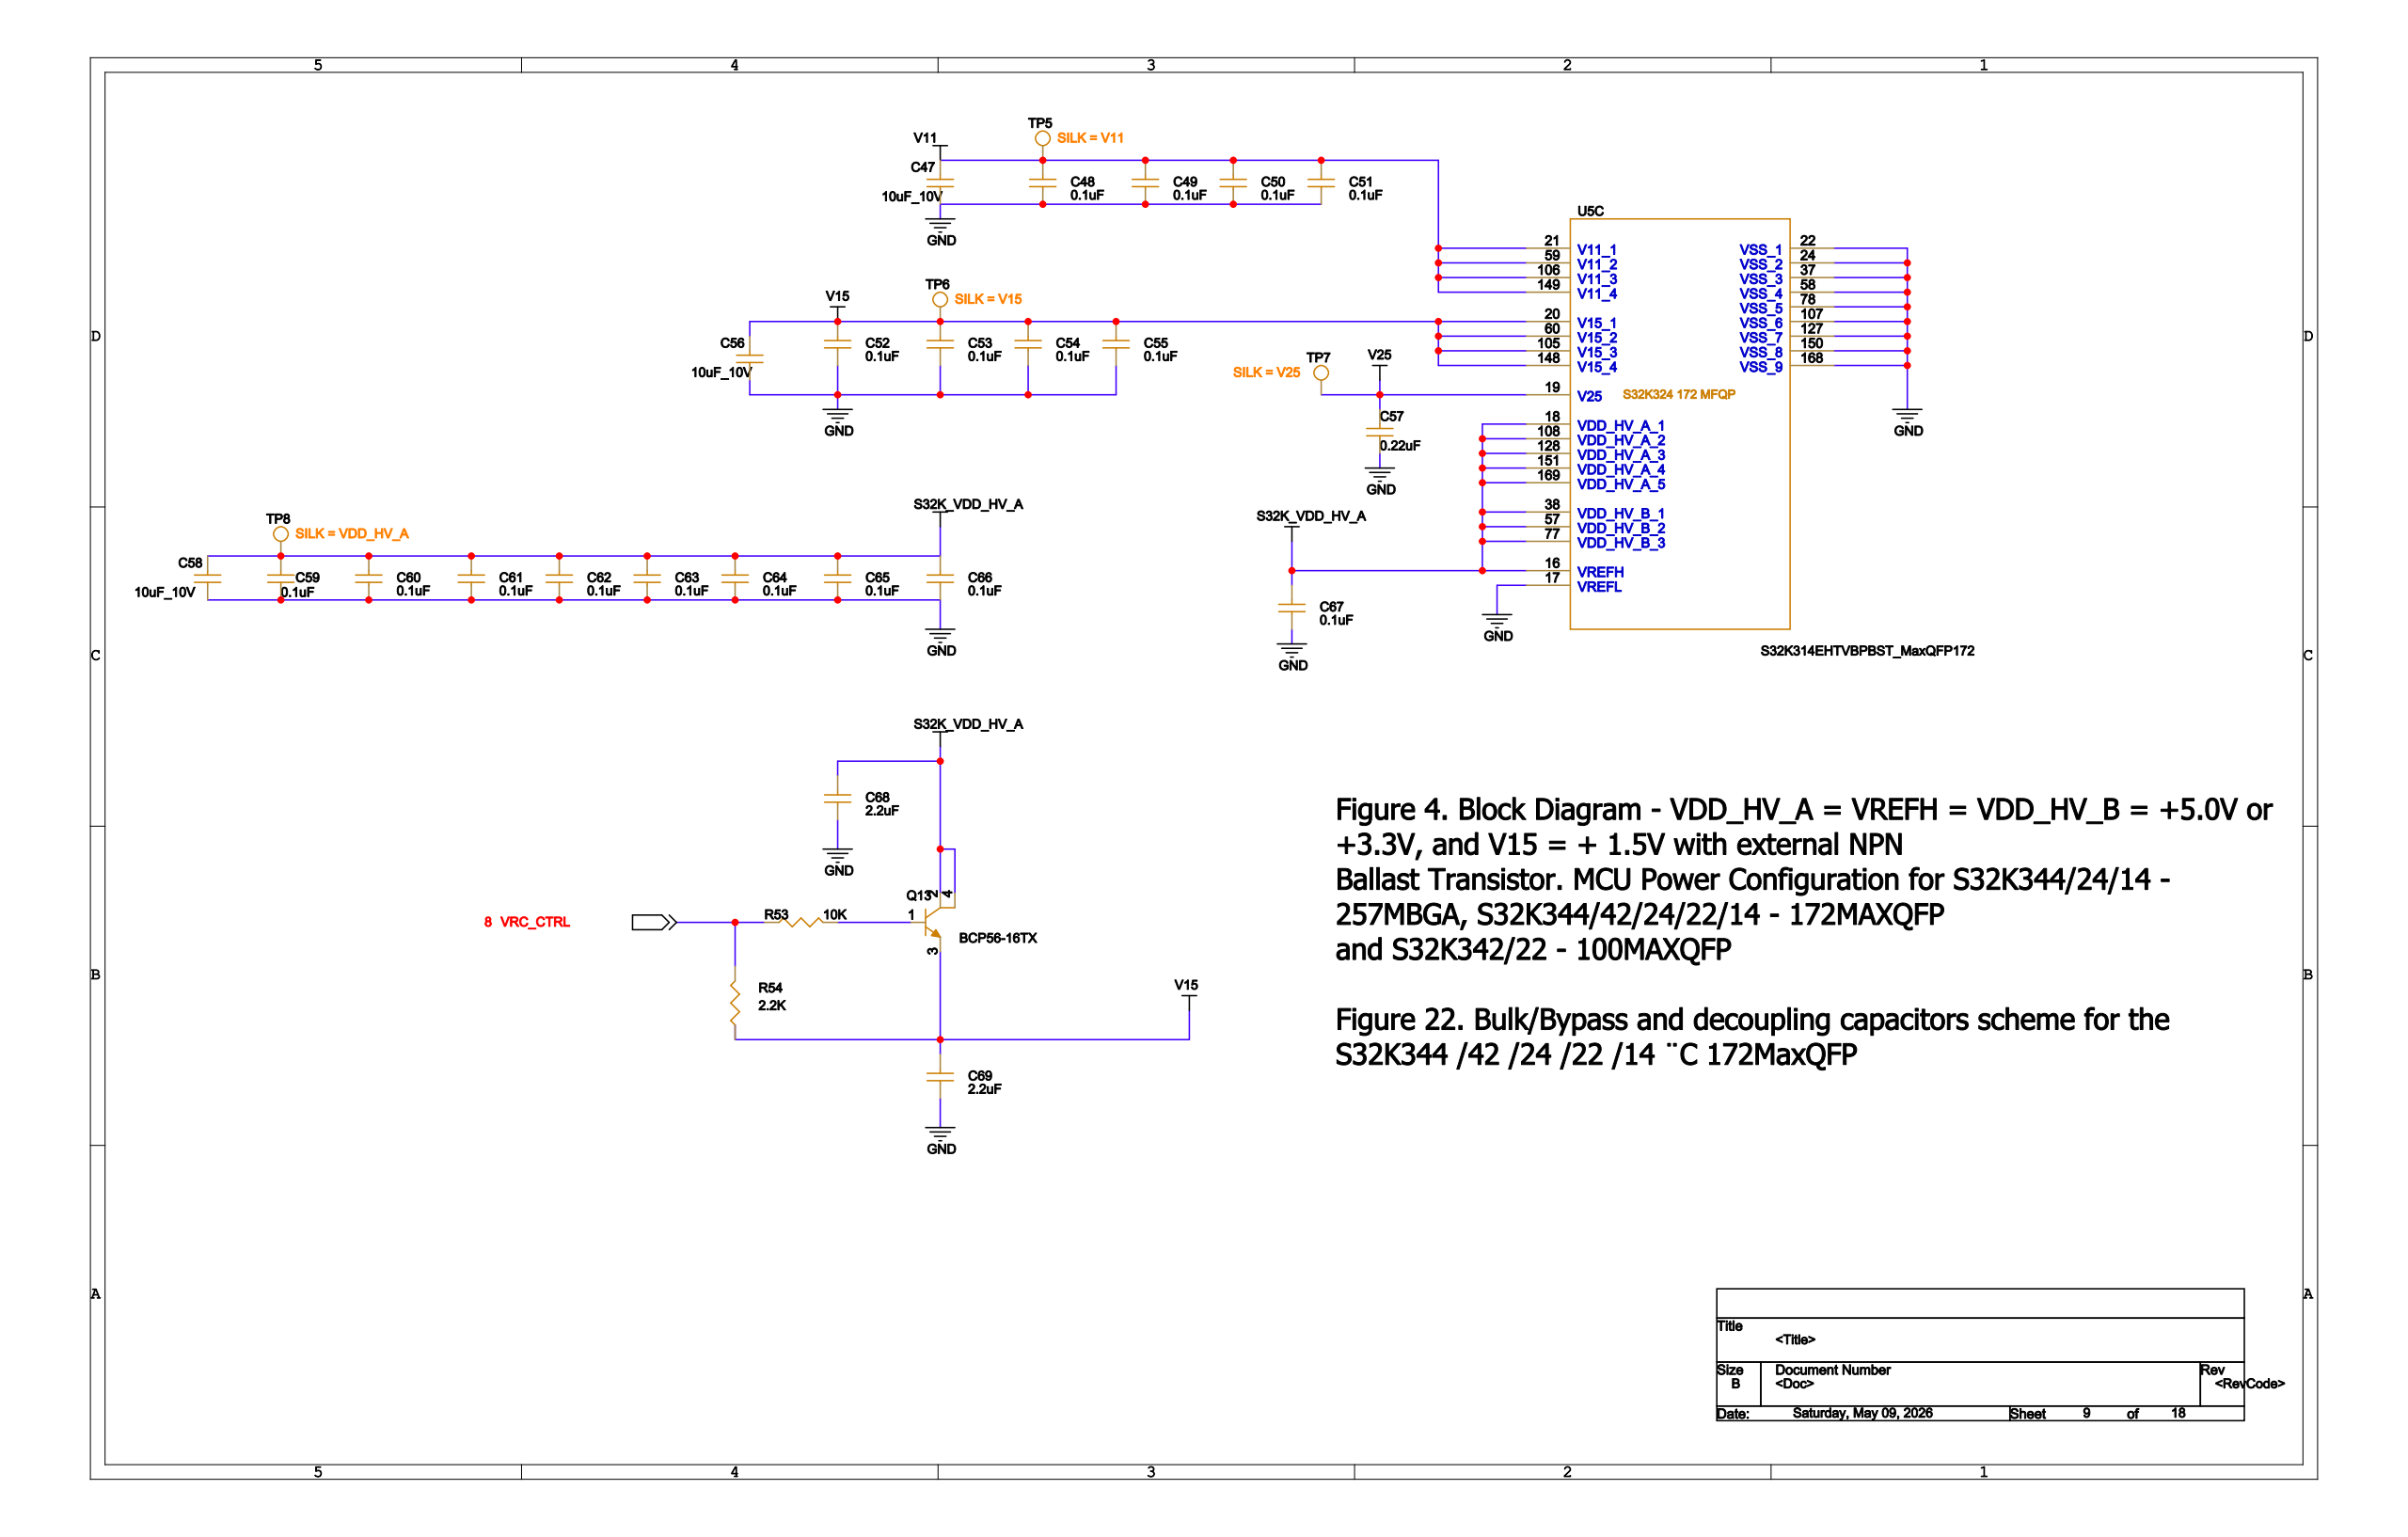Circuit board | Cadence Allegro | 330 parts | 215 nets | one sheet of the schematic
Parts on this sheet (reference | value | footprint):
C47 | 10uF_10V | 0603
C48 | 0.1uF | 0402
C49 | 0.1uF | 0402
C50 | 0.1uF | 0402
C51 | 0.1uF | 0402
C52 | 0.1uF | 0402
C53 | 0.1uF | 0402
C54 | 0.1uF | 0402
C55 | 0.1uF | 0402
C56 | 10uF_10V | 0603
C57 | 0.22uF | 0402
C58 | 10uF_10V | 0603
C59 | 0.1uF | 0402
C60 | 0.1uF | 0402
C61 | 0.1uF | 0402
C62 | 0.1uF | 0402
C63 | 0.1uF | 0402
C64 | 0.1uF | 0402
C65 | 0.1uF | 0402
C66 | 0.1uF | 0402
C67 | 0.1uF | 0402
C68 | 2.2uF | 0402
C69 | 2.2uF | 0402
Q13 | BCP56-16TX | BCP56_SOT-223
R53 | 10K | 0402
R54 | 2.2K | 0402
TP5 | TP | S0400CI
TP6 | TP | S0400CI
TP7 | TP | S0400CI
TP8 | TP | S0400CI
U5 | S32K314EHTVBPBST_MaxQFP172 | MQFP172_0P65_16X16
Nets of these parts (net: part-pin ...):
GND: C47-1 C48-1 C49-1 C50-1 C51-1 C52-1 C53-1 C54-1 C55-1 C56-1 C57-1 C58-1 C59-1 C60-1 C61-1 C62-1 C63-1 C64-1 C65-1 C66-1 C67-1 C68-1 C69-1 U5-17 U5-22 U5-24 U5-37 U5-58 U5-78 U5-107 U5-127 U5-150 U5-168
V11: C47-2 C48-2 C49-2 C50-2 C51-2 TP5-1 U5-21 U5-59 U5-106 U5-149
V15: C52-2 C53-2 C54-2 C55-2 C56-2 C69-2 Q13-3 R54-1 TP6-1 U5-20 U5-60 U5-105 U5-148
S32K_VDD_HV_A: C58-2 C59-2 C60-2 C61-2 C62-2 C63-2 C64-2 C65-2 C66-2 C67-2 C68-2 Q13-2 Q13-4 TP8-1 U5-16 U5-18 U5-38 U5-57 U5-77 U5-108 U5-128 U5-151 U5-169
VRC_CTRL: R53-1 R54-2
N1673456: Q13-1 R53-2
V25: C57-2 TP7-1 U5-19